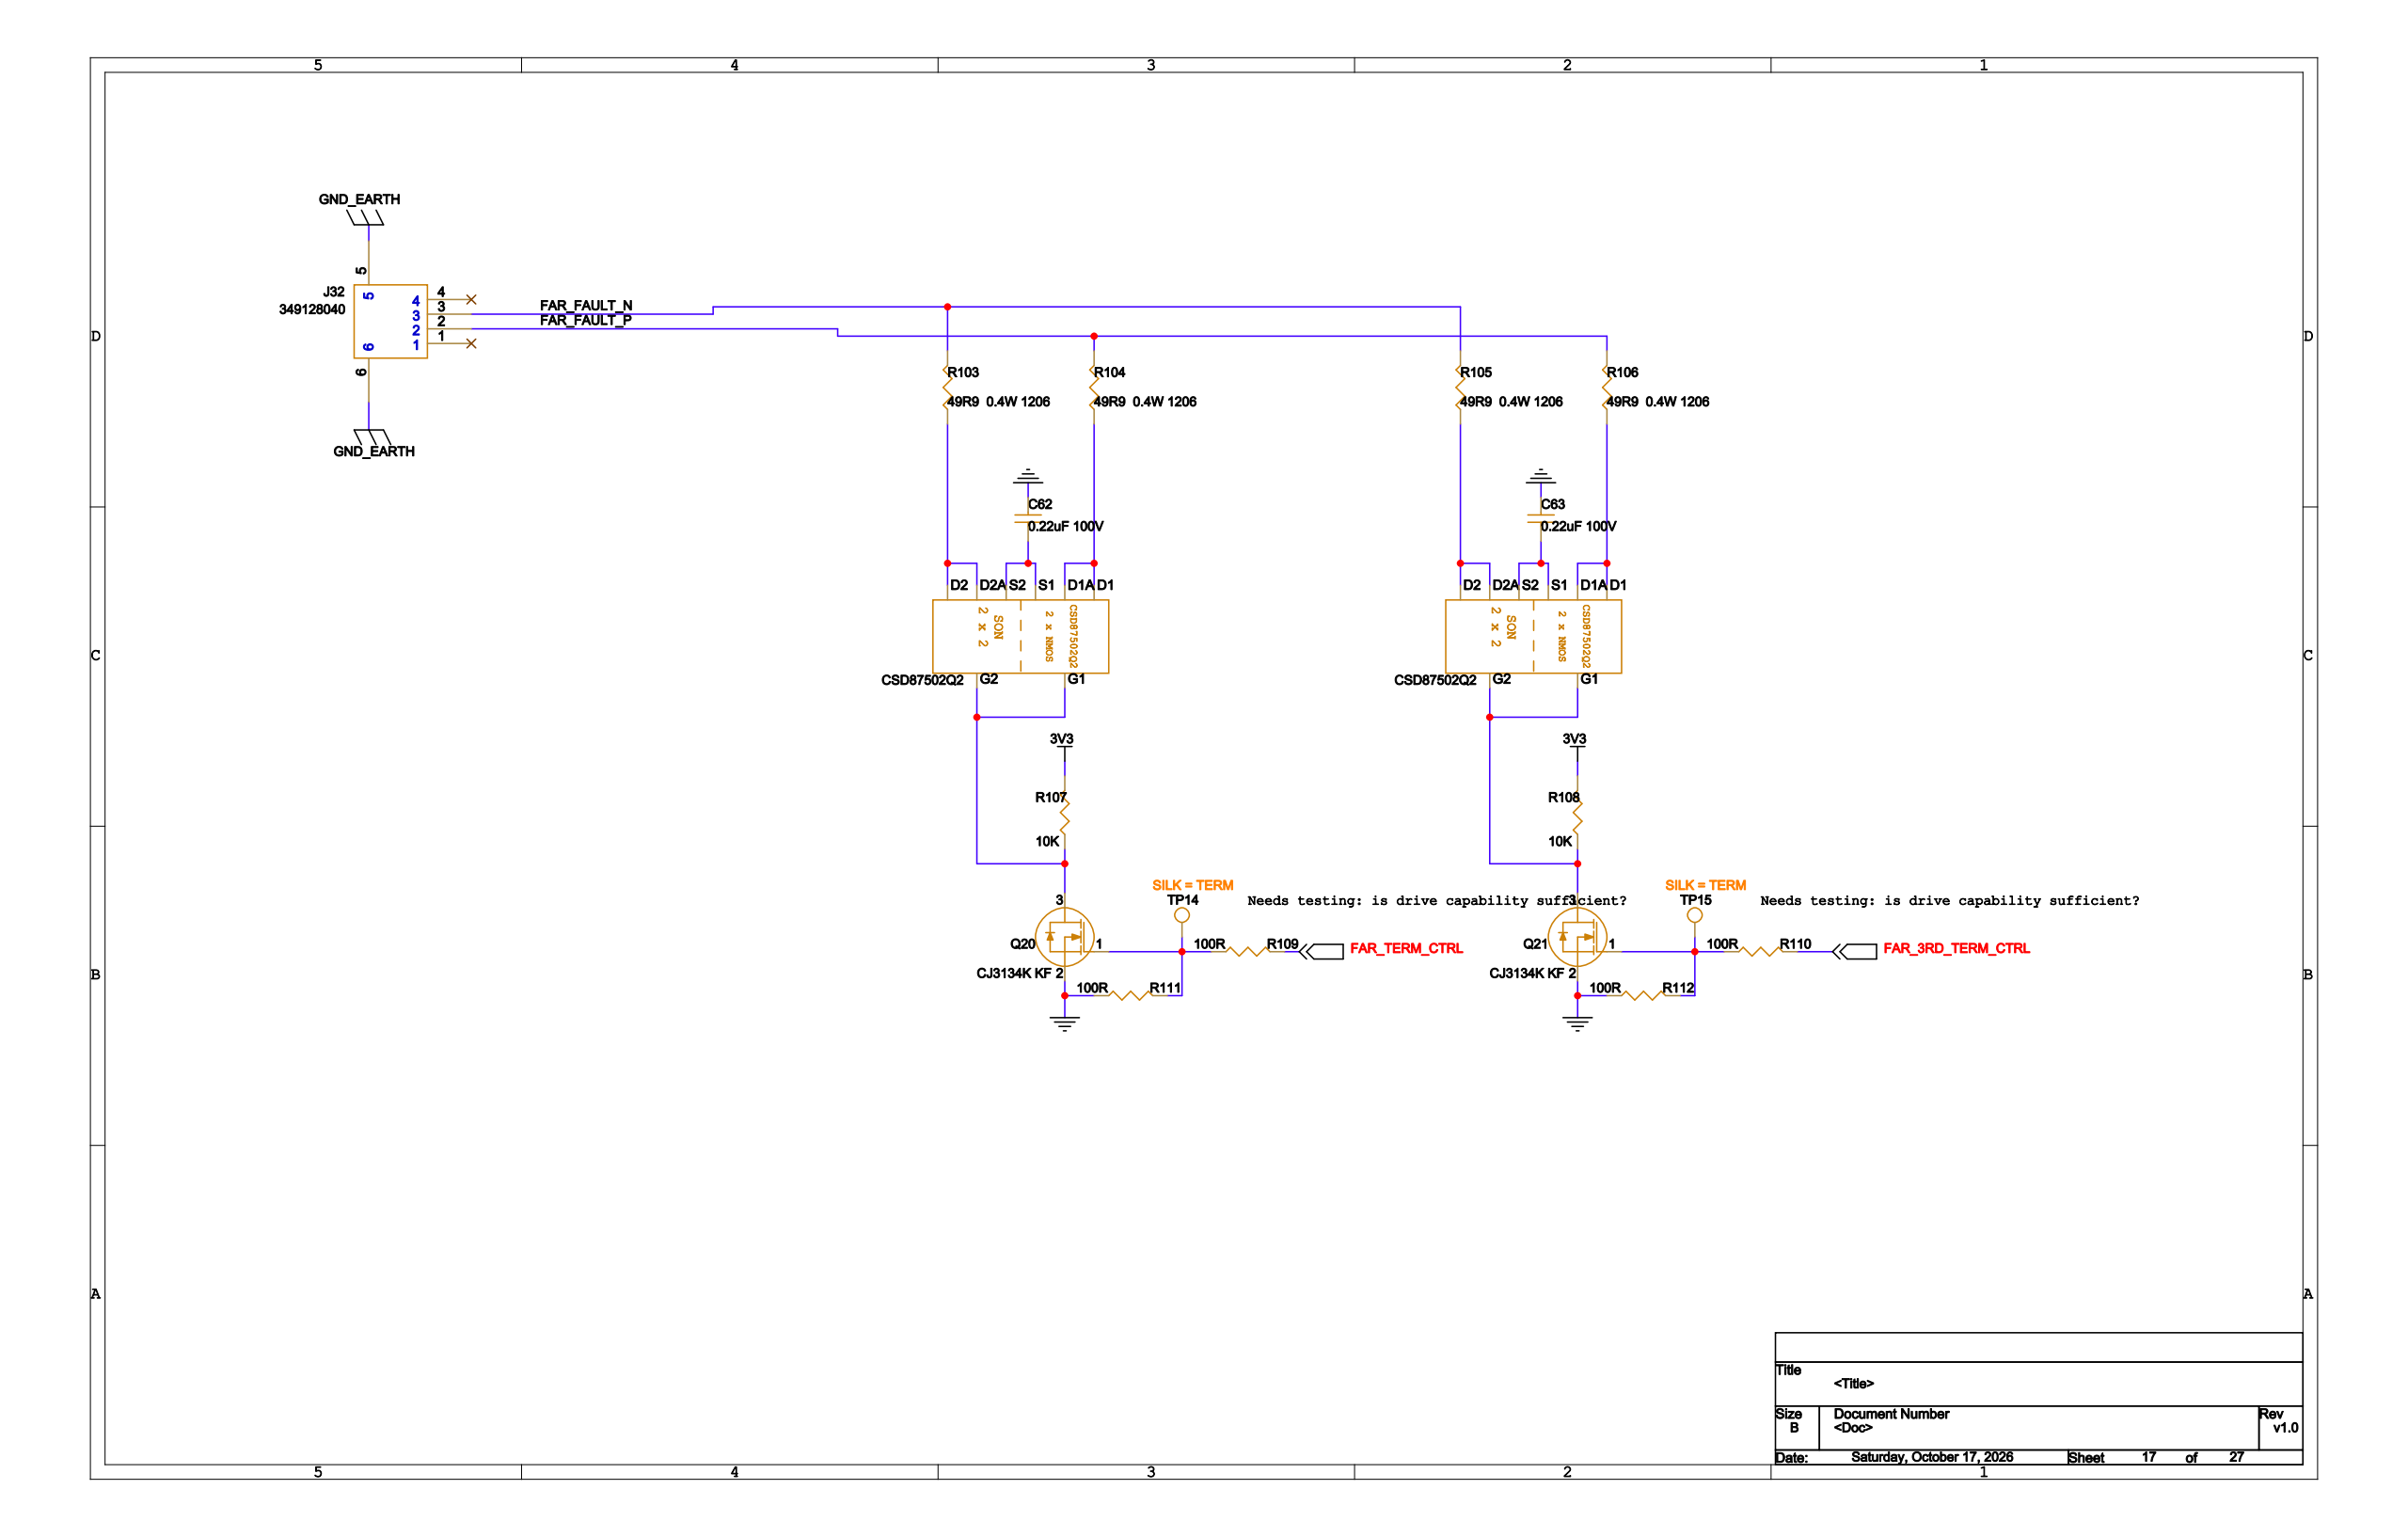Circuit board | Cadence Allegro | 477 parts | 327 nets | one sheet of the schematic
Parts on this sheet (reference | value | footprint):
C62 | 0.22uF 100V | 0805
C63 | 0.22uF 100V | 0805
J32 | 349128040 | 349128040
Q20 | CJ3134K KF | SOT723
Q21 | CJ3134K KF | SOT723
R103 | 49R9  0.4W 1206 | 1206
R104 | 49R9  0.4W 1206 | 1206
R105 | 49R9  0.4W 1206 | 1206
R106 | 49R9  0.4W 1206 | 1206
R107 | 10K | 0402
R108 | 10K | 0402
R109 | 100R | 0402
R110 | 100R | 0402
R111 | 100R | 0402
R112 | 100R | 0402
TP14 | TP | S0400CI
TP15 | TP | S0400CI
Nets of these parts (net: part-pin ...):
GND: C62-1 C63-1 Q20-2 Q21-2 R111-2 R112-2
FAR_FAULT_N: J32-3 R103-1 R105-1
N16838641: R103-2
FAR_FAULT_P: J32-2 R104-1 R106-1
N16838643: R104-2
N16838645: R105-2
N16838647: R106-2
3V3: R107-2 R108-2
GND_EARTH: J32-5 J32-6
N16838739: Q20-3 R107-1
N16838743: Q21-3 R108-1
FAR_TERM_CTRL: R109-1
FAR_3RD_TERM_CTRL: R110-1
N16838673: C62-2
N16838675: C63-2
N16838841: Q20-1 R109-2 R111-1 TP14-1
N16838856: Q21-1 R110-2 R112-1 TP15-1